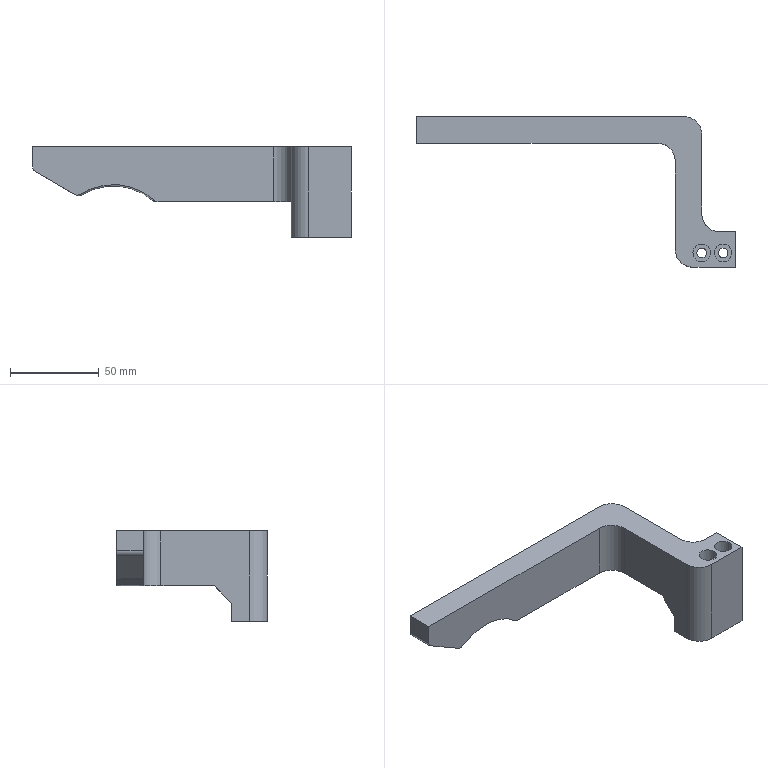Part | NX | 1 solid | 31 faces | box 180 x 85 x 51 mm | volume 114563 mm3 | plane 18 | cylinder 10 | spline 2 | cone 1 | commonest cylinder face diameters 20 x4 5.5 x2 10 x2 6 x1 12.2 x1
STEP:
#1=CARTESIAN_POINT('',(-63.096,27.5,-26.764));
#2=VERTEX_POINT('',#1);
#3=CARTESIAN_POINT('',(-21.145,27.5,-30.228));
#4=VERTEX_POINT('',#3);
#5=CARTESIAN_POINT('',(-44.4,27.5,-56.099));
#6=DIRECTION('',(0.,-1.,0.));
#7=DIRECTION('',(1.,0.,0.));
#8=AXIS2_PLACEMENT_3D('',#5,#6,#7);
#9=CIRCLE('',#8,34.786);
#10=EDGE_CURVE('',#2,#4,#9,.F.);
#11=ORIENTED_EDGE('',*,*,#10,.T.);
#12=CARTESIAN_POINT('',(-19.13,27.5,-31.));
#13=VERTEX_POINT('',#12);
#14=CARTESIAN_POINT('',(-21.145,27.5,-30.228));
#15=CARTESIAN_POINT('',(-20.592,27.5,-30.725));
#16=CARTESIAN_POINT('',(-19.874,27.5,-31.));
#17=CARTESIAN_POINT('',(-19.13,27.5,-31.));
#18=B_SPLINE_CURVE_WITH_KNOTS('',3,(#14,#15,#16,#17),.UNSPECIFIED.,.F.,.F.,(4,4),(0.,0.002195),.UNSPECIFIED.);
#19=EDGE_CURVE('',#4,#13,#18,.T.);
#20=ORIENTED_EDGE('',*,*,#19,.T.);
#21=CARTESIAN_POINT('',(46.,27.5,-31.));
#22=VERTEX_POINT('',#21);
#23=CARTESIAN_POINT('',(-90.,27.5,-31.));
#24=DIRECTION('',(1.,0.,0.));
#25=VECTOR('',#24,1000.);
#26=LINE('',#23,#25);
#27=EDGE_CURVE('',#22,#13,#26,.F.);
#28=ORIENTED_EDGE('',*,*,#27,.F.);
#29=CARTESIAN_POINT('',(46.,27.5,0.));
#30=VERTEX_POINT('',#29);
#31=CARTESIAN_POINT('',(46.,27.5,-31.));
#32=DIRECTION('',(0.,0.,1.));
#33=VECTOR('',#32,1000.);
#34=LINE('',#31,#33);
#35=EDGE_CURVE('',#30,#22,#34,.F.);
#36=ORIENTED_EDGE('',*,*,#35,.F.);
#37=CARTESIAN_POINT('',(-90.,27.5,0.));
#38=VERTEX_POINT('',#37);
#39=CARTESIAN_POINT('',(-20.212,27.5,0.));
#40=DIRECTION('',(1.,0.,0.));
#41=VECTOR('',#40,1000.);
#42=LINE('',#39,#41);
#43=EDGE_CURVE('',#30,#38,#42,.F.);
#44=ORIENTED_EDGE('',*,*,#43,.T.);
#45=CARTESIAN_POINT('',(-90.,27.5,-11.367));
#46=VERTEX_POINT('',#45);
#47=CARTESIAN_POINT('',(-90.,27.5,-31.));
#48=DIRECTION('',(0.,0.,1.));
#49=VECTOR('',#48,1000.);
#50=LINE('',#47,#49);
#51=EDGE_CURVE('',#38,#46,#50,.F.);
#52=ORIENTED_EDGE('',*,*,#51,.T.);
#53=CARTESIAN_POINT('',(-88.5,27.5,-13.965));
#54=VERTEX_POINT('',#53);
#55=CARTESIAN_POINT('',(-87.,27.5,-11.367));
#56=DIRECTION('',(0.,-1.,0.));
#57=DIRECTION('',(1.,0.,0.));
#58=AXIS2_PLACEMENT_3D('',#55,#56,#57);
#59=CIRCLE('',#58,3.);
#60=EDGE_CURVE('',#46,#54,#59,.T.);
#61=ORIENTED_EDGE('',*,*,#60,.T.);
#62=CARTESIAN_POINT('',(-66.215,27.5,-26.831));
#63=VERTEX_POINT('',#62);
#64=CARTESIAN_POINT('',(-29.907,27.5,-47.793));
#65=DIRECTION('',(0.866,0.,-0.5));
#66=VECTOR('',#65,1000.);
#67=LINE('',#64,#66);
#68=EDGE_CURVE('',#54,#63,#67,.T.);
#69=ORIENTED_EDGE('',*,*,#68,.T.);
#70=CARTESIAN_POINT('',(-66.215,27.5,-26.831));
#71=CARTESIAN_POINT('',(-65.26,27.5,-27.383));
#72=CARTESIAN_POINT('',(-64.026,27.5,-27.357));
#73=CARTESIAN_POINT('',(-63.096,27.5,-26.764));
#74=B_SPLINE_CURVE_WITH_KNOTS('',3,(#70,#71,#72,#73),.UNSPECIFIED.,.F.,.F.,(4,4),(0.,0.003262),.UNSPECIFIED.);
#75=EDGE_CURVE('',#63,#2,#74,.T.);
#76=ORIENTED_EDGE('',*,*,#75,.T.);
#77=EDGE_LOOP('',(#11,#20,#28,#36,#44,#52,#61,#69,#76));
#78=FACE_BOUND('',#77,.T.);
#79=CARTESIAN_POINT('',(-20.212,27.5,-31.));
#80=DIRECTION('',(0.,-1.,0.));
#81=DIRECTION('',(0.,0.,-1.));
#82=AXIS2_PLACEMENT_3D('',#79,#80,#81);
#83=PLANE('',#82);
#84=ADVANCED_FACE('',(#78),#83,.T.);
#85=CARTESIAN_POINT('',(-20.322,42.5,-31.));
#86=VERTEX_POINT('',#85);
#87=CARTESIAN_POINT('',(61.,42.5,-31.));
#88=VERTEX_POINT('',#87);
#89=CARTESIAN_POINT('',(61.,42.5,-31.));
#90=DIRECTION('',(-1.,0.,0.));
#91=VECTOR('',#90,1000.);
#92=LINE('',#89,#91);
#93=EDGE_CURVE('',#86,#88,#92,.F.);
#94=ORIENTED_EDGE('',*,*,#93,.F.);
#95=CARTESIAN_POINT('',(-22.283,42.5,-30.275));
#96=VERTEX_POINT('',#95);
#97=CARTESIAN_POINT('',(-20.322,42.5,-31.));
#98=CARTESIAN_POINT('',(-21.041,42.5,-31.));
#99=CARTESIAN_POINT('',(-21.737,42.5,-30.743));
#100=CARTESIAN_POINT('',(-22.283,42.5,-30.275));
#101=B_SPLINE_CURVE_WITH_KNOTS('',3,(#97,#98,#99,#100),.UNSPECIFIED.,.F.,.F.,(4,4),(0.,0.002124),.UNSPECIFIED.);
#102=EDGE_CURVE('',#86,#96,#101,.T.);
#103=ORIENTED_EDGE('',*,*,#102,.T.);
#104=CARTESIAN_POINT('',(-62.355,42.5,-27.226));
#105=VERTEX_POINT('',#104);
#106=CARTESIAN_POINT('',(-44.4,42.5,-56.099));
#107=DIRECTION('',(0.,1.,0.));
#108=DIRECTION('',(-1.,0.,0.));
#109=AXIS2_PLACEMENT_3D('',#106,#107,#108);
#110=CIRCLE('',#109,34.);
#111=EDGE_CURVE('',#96,#105,#110,.F.);
#112=ORIENTED_EDGE('',*,*,#111,.T.);
#113=CARTESIAN_POINT('',(-65.445,42.5,-27.276));
#114=VERTEX_POINT('',#113);
#115=CARTESIAN_POINT('',(-62.355,42.5,-27.226));
#116=CARTESIAN_POINT('',(-63.282,42.5,-27.803));
#117=CARTESIAN_POINT('',(-64.5,42.5,-27.822));
#118=CARTESIAN_POINT('',(-65.445,42.5,-27.276));
#119=B_SPLINE_CURVE_WITH_KNOTS('',3,(#115,#116,#117,#118),.UNSPECIFIED.,.F.,.F.,(4,4),(0.,0.003229),.UNSPECIFIED.);
#120=EDGE_CURVE('',#105,#114,#119,.T.);
#121=ORIENTED_EDGE('',*,*,#120,.T.);
#122=CARTESIAN_POINT('',(-88.5,42.5,-13.965));
#123=VERTEX_POINT('',#122);
#124=CARTESIAN_POINT('',(-66.211,42.5,-26.834));
#125=DIRECTION('',(-0.866,0.,0.5));
#126=VECTOR('',#125,1000.);
#127=LINE('',#124,#126);
#128=EDGE_CURVE('',#114,#123,#127,.T.);
#129=ORIENTED_EDGE('',*,*,#128,.T.);
#130=CARTESIAN_POINT('',(-90.,42.5,-11.367));
#131=VERTEX_POINT('',#130);
#132=CARTESIAN_POINT('',(-87.,42.5,-11.367));
#133=DIRECTION('',(0.,1.,0.));
#134=DIRECTION('',(1.,0.,0.));
#135=AXIS2_PLACEMENT_3D('',#132,#133,#134);
#136=CIRCLE('',#135,3.);
#137=EDGE_CURVE('',#123,#131,#136,.T.);
#138=ORIENTED_EDGE('',*,*,#137,.T.);
#139=CARTESIAN_POINT('',(-90.,42.5,0.));
#140=VERTEX_POINT('',#139);
#141=CARTESIAN_POINT('',(-90.,42.5,-31.));
#142=DIRECTION('',(0.,0.,1.));
#143=VECTOR('',#142,1000.);
#144=LINE('',#141,#143);
#145=EDGE_CURVE('',#140,#131,#144,.F.);
#146=ORIENTED_EDGE('',*,*,#145,.F.);
#147=CARTESIAN_POINT('',(61.,42.5,0.));
#148=VERTEX_POINT('',#147);
#149=CARTESIAN_POINT('',(-88.5,42.5,0.));
#150=DIRECTION('',(-1.,0.,0.));
#151=VECTOR('',#150,1000.);
#152=LINE('',#149,#151);
#153=EDGE_CURVE('',#140,#148,#152,.F.);
#154=ORIENTED_EDGE('',*,*,#153,.T.);
#155=CARTESIAN_POINT('',(61.,42.5,-31.));
#156=DIRECTION('',(0.,0.,1.));
#157=VECTOR('',#156,1000.);
#158=LINE('',#155,#157);
#159=EDGE_CURVE('',#148,#88,#158,.F.);
#160=ORIENTED_EDGE('',*,*,#159,.T.);
#161=EDGE_LOOP('',(#94,#103,#112,#121,#129,#138,#146,#154,#160));
#162=FACE_BOUND('',#161,.T.);
#163=CARTESIAN_POINT('',(-88.5,42.5,-31.));
#164=DIRECTION('',(0.,1.,0.));
#165=DIRECTION('',(0.,0.,1.));
#166=AXIS2_PLACEMENT_3D('',#163,#164,#165);
#167=PLANE('',#166);
#168=ADVANCED_FACE('',(#162),#167,.T.);
#169=CARTESIAN_POINT('',(71.,32.5,-31.));
#170=VERTEX_POINT('',#169);
#171=CARTESIAN_POINT('',(71.,-12.5,-31.));
#172=VERTEX_POINT('',#171);
#173=CARTESIAN_POINT('',(71.,-12.5,-31.));
#174=DIRECTION('',(0.,1.,0.));
#175=VECTOR('',#174,1000.);
#176=LINE('',#173,#175);
#177=EDGE_CURVE('',#170,#172,#176,.F.);
#178=ORIENTED_EDGE('',*,*,#177,.T.);
#179=CARTESIAN_POINT('',(56.,-12.5,-31.));
#180=VERTEX_POINT('',#179);
#181=CARTESIAN_POINT('',(46.,-12.5,-31.));
#182=DIRECTION('',(-1.,0.,0.));
#183=VECTOR('',#182,1000.);
#184=LINE('',#181,#183);
#185=EDGE_CURVE('',#172,#180,#184,.T.);
#186=ORIENTED_EDGE('',*,*,#185,.T.);
#187=CARTESIAN_POINT('',(56.,17.5,-31.));
#188=VERTEX_POINT('',#187);
#189=CARTESIAN_POINT('',(56.,17.5,-31.));
#190=DIRECTION('',(0.,-1.,0.));
#191=VECTOR('',#190,1000.);
#192=LINE('',#189,#191);
#193=EDGE_CURVE('',#180,#188,#192,.F.);
#194=ORIENTED_EDGE('',*,*,#193,.T.);
#195=CARTESIAN_POINT('',(46.,17.5,-31.));
#196=DIRECTION('',(0.,0.,-1.));
#197=DIRECTION('',(1.,0.,0.));
#198=AXIS2_PLACEMENT_3D('',#195,#196,#197);
#199=CIRCLE('',#198,10.);
#200=EDGE_CURVE('',#188,#22,#199,.F.);
#201=ORIENTED_EDGE('',*,*,#200,.T.);
#202=ORIENTED_EDGE('',*,*,#27,.T.);
#203=CARTESIAN_POINT('',(-19.13,27.5,-31.));
#204=CARTESIAN_POINT('',(-19.522,32.5,-31.));
#205=CARTESIAN_POINT('',(-19.919,37.5,-31.));
#206=CARTESIAN_POINT('',(-20.322,42.5,-31.));
#207=B_SPLINE_CURVE_WITH_KNOTS('',3,(#203,#204,#205,#206),.UNSPECIFIED.,.F.,.F.,(4,4),(0.,0.01505),.UNSPECIFIED.);
#208=EDGE_CURVE('',#13,#86,#207,.T.);
#209=ORIENTED_EDGE('',*,*,#208,.T.);
#210=ORIENTED_EDGE('',*,*,#93,.T.);
#211=CARTESIAN_POINT('',(61.,32.5,-31.));
#212=DIRECTION('',(0.,0.,1.));
#213=DIRECTION('',(1.,0.,0.));
#214=AXIS2_PLACEMENT_3D('',#211,#212,#213);
#215=CIRCLE('',#214,10.);
#216=EDGE_CURVE('',#88,#170,#215,.F.);
#217=ORIENTED_EDGE('',*,*,#216,.T.);
#218=EDGE_LOOP('',(#178,#186,#194,#201,#202,#209,#210,#217));
#219=FACE_BOUND('',#218,.T.);
#220=CARTESIAN_POINT('',(46.,17.5,-31.));
#221=DIRECTION('',(0.,0.,-1.));
#222=DIRECTION('',(1.,0.,0.));
#223=AXIS2_PLACEMENT_3D('',#220,#221,#222);
#224=PLANE('',#223);
#225=ADVANCED_FACE('',(#219),#224,.T.);
#226=CARTESIAN_POINT('',(56.,17.5,0.));
#227=VERTEX_POINT('',#226);
#228=CARTESIAN_POINT('',(46.,17.5,0.));
#229=DIRECTION('',(0.,0.,-1.));
#230=DIRECTION('',(1.,0.,0.));
#231=AXIS2_PLACEMENT_3D('',#228,#229,#230);
#232=CIRCLE('',#231,10.);
#233=EDGE_CURVE('',#227,#30,#232,.F.);
#234=ORIENTED_EDGE('',*,*,#233,.T.);
#235=ORIENTED_EDGE('',*,*,#35,.T.);
#236=ORIENTED_EDGE('',*,*,#200,.F.);
#237=CARTESIAN_POINT('',(56.,17.5,-31.));
#238=DIRECTION('',(0.,0.,1.));
#239=VECTOR('',#238,1000.);
#240=LINE('',#237,#239);
#241=EDGE_CURVE('',#227,#188,#240,.F.);
#242=ORIENTED_EDGE('',*,*,#241,.F.);
#243=EDGE_LOOP('',(#234,#235,#236,#242));
#244=FACE_BOUND('',#243,.T.);
#245=CARTESIAN_POINT('',(46.,17.5,-31.));
#246=DIRECTION('',(0.,0.,1.));
#247=DIRECTION('',(-1.,0.,0.));
#248=AXIS2_PLACEMENT_3D('',#245,#246,#247);
#249=CYLINDRICAL_SURFACE('',#248,10.);
#250=ADVANCED_FACE('',(#244),#249,.F.);
#251=CARTESIAN_POINT('',(56.,-32.5,0.));
#252=VERTEX_POINT('',#251);
#253=CARTESIAN_POINT('',(56.,-12.5,0.));
#254=DIRECTION('',(0.,-1.,0.));
#255=VECTOR('',#254,1000.);
#256=LINE('',#253,#255);
#257=EDGE_CURVE('',#252,#227,#256,.F.);
#258=ORIENTED_EDGE('',*,*,#257,.T.);
#259=ORIENTED_EDGE('',*,*,#241,.T.);
#260=ORIENTED_EDGE('',*,*,#193,.F.);
#261=CARTESIAN_POINT('',(56.,-22.5,-41.));
#262=VERTEX_POINT('',#261);
#263=CARTESIAN_POINT('',(56.,-12.5,-31.));
#264=DIRECTION('',(0.,-0.7071,-0.7071));
#265=VECTOR('',#264,1000.);
#266=LINE('',#263,#265);
#267=EDGE_CURVE('',#180,#262,#266,.T.);
#268=ORIENTED_EDGE('',*,*,#267,.T.);
#269=CARTESIAN_POINT('',(56.,-22.5,-51.));
#270=VERTEX_POINT('',#269);
#271=CARTESIAN_POINT('',(56.,-22.5,-51.));
#272=DIRECTION('',(0.,0.,1.));
#273=VECTOR('',#272,1000.);
#274=LINE('',#271,#273);
#275=EDGE_CURVE('',#270,#262,#274,.T.);
#276=ORIENTED_EDGE('',*,*,#275,.F.);
#277=CARTESIAN_POINT('',(56.,-32.5,-51.));
#278=VERTEX_POINT('',#277);
#279=CARTESIAN_POINT('',(56.,-32.5,-51.));
#280=DIRECTION('',(0.,1.,0.));
#281=VECTOR('',#280,1000.);
#282=LINE('',#279,#281);
#283=EDGE_CURVE('',#278,#270,#282,.T.);
#284=ORIENTED_EDGE('',*,*,#283,.F.);
#285=CARTESIAN_POINT('',(56.,-32.5,-51.));
#286=DIRECTION('',(0.,0.,1.));
#287=VECTOR('',#286,1000.);
#288=LINE('',#285,#287);
#289=EDGE_CURVE('',#278,#252,#288,.T.);
#290=ORIENTED_EDGE('',*,*,#289,.T.);
#291=EDGE_LOOP('',(#258,#259,#260,#268,#276,#284,#290));
#292=FACE_BOUND('',#291,.T.);
#293=CARTESIAN_POINT('',(56.,-12.5,-31.));
#294=DIRECTION('',(-1.,0.,0.));
#295=DIRECTION('',(0.,0.,-1.));
#296=AXIS2_PLACEMENT_3D('',#293,#294,#295);
#297=PLANE('',#296);
#298=ADVANCED_FACE('',(#292),#297,.T.);
#299=CARTESIAN_POINT('',(71.,-12.5,0.));
#300=VERTEX_POINT('',#299);
#301=CARTESIAN_POINT('',(81.,-22.5,0.));
#302=VERTEX_POINT('',#301);
#303=CARTESIAN_POINT('',(81.,-12.5,0.));
#304=DIRECTION('',(0.,0.,-1.));
#305=DIRECTION('',(1.,0.,0.));
#306=AXIS2_PLACEMENT_3D('',#303,#304,#305);
#307=CIRCLE('',#306,10.);
#308=EDGE_CURVE('',#300,#302,#307,.F.);
#309=ORIENTED_EDGE('',*,*,#308,.T.);
#310=CARTESIAN_POINT('',(81.,-22.5,-41.));
#311=VERTEX_POINT('',#310);
#312=CARTESIAN_POINT('',(81.,-22.5,-31.));
#313=DIRECTION('',(0.,0.,1.));
#314=VECTOR('',#313,1000.);
#315=LINE('',#312,#314);
#316=EDGE_CURVE('',#302,#311,#315,.F.);
#317=ORIENTED_EDGE('',*,*,#316,.T.);
#318=CARTESIAN_POINT('',(81.,-12.5,-31.));
#319=DIRECTION('',(0.,-0.7071,0.7071));
#320=DIRECTION('',(0.,0.7071,0.7071));
#321=AXIS2_PLACEMENT_3D('',#318,#319,#320);
#322=ELLIPSE('',#321,14.142,10.);
#323=EDGE_CURVE('',#311,#172,#322,.F.);
#324=ORIENTED_EDGE('',*,*,#323,.T.);
#325=CARTESIAN_POINT('',(71.,-12.5,-31.));
#326=DIRECTION('',(0.,0.,1.));
#327=VECTOR('',#326,1000.);
#328=LINE('',#325,#327);
#329=EDGE_CURVE('',#300,#172,#328,.F.);
#330=ORIENTED_EDGE('',*,*,#329,.F.);
#331=EDGE_LOOP('',(#309,#317,#324,#330));
#332=FACE_BOUND('',#331,.T.);
#333=CARTESIAN_POINT('',(81.,-12.5,-31.));
#334=DIRECTION('',(0.,0.,1.));
#335=DIRECTION('',(-1.,0.,0.));
#336=AXIS2_PLACEMENT_3D('',#333,#334,#335);
#337=CYLINDRICAL_SURFACE('',#336,10.);
#338=ADVANCED_FACE('',(#332),#337,.F.);
#339=CARTESIAN_POINT('',(71.,32.5,0.));
#340=VERTEX_POINT('',#339);
#341=CARTESIAN_POINT('',(71.,-12.5,0.));
#342=DIRECTION('',(0.,1.,0.));
#343=VECTOR('',#342,1000.);
#344=LINE('',#341,#343);
#345=EDGE_CURVE('',#340,#300,#344,.F.);
#346=ORIENTED_EDGE('',*,*,#345,.T.);
#347=ORIENTED_EDGE('',*,*,#329,.T.);
#348=ORIENTED_EDGE('',*,*,#177,.F.);
#349=CARTESIAN_POINT('',(71.,32.5,-31.));
#350=DIRECTION('',(0.,0.,1.));
#351=VECTOR('',#350,1000.);
#352=LINE('',#349,#351);
#353=EDGE_CURVE('',#340,#170,#352,.F.);
#354=ORIENTED_EDGE('',*,*,#353,.F.);
#355=EDGE_LOOP('',(#346,#347,#348,#354));
#356=FACE_BOUND('',#355,.T.);
#357=CARTESIAN_POINT('',(71.,-12.5,-31.));
#358=DIRECTION('',(1.,0.,0.));
#359=DIRECTION('',(0.,0.,1.));
#360=AXIS2_PLACEMENT_3D('',#357,#358,#359);
#361=PLANE('',#360);
#362=ADVANCED_FACE('',(#356),#361,.T.);
#363=CARTESIAN_POINT('',(61.,32.5,0.));
#364=DIRECTION('',(0.,0.,1.));
#365=DIRECTION('',(1.,0.,0.));
#366=AXIS2_PLACEMENT_3D('',#363,#364,#365);
#367=CIRCLE('',#366,10.);
#368=EDGE_CURVE('',#148,#340,#367,.F.);
#369=ORIENTED_EDGE('',*,*,#368,.T.);
#370=ORIENTED_EDGE('',*,*,#353,.T.);
#371=ORIENTED_EDGE('',*,*,#216,.F.);
#372=ORIENTED_EDGE('',*,*,#159,.F.);
#373=EDGE_LOOP('',(#369,#370,#371,#372));
#374=FACE_BOUND('',#373,.T.);
#375=CARTESIAN_POINT('',(61.,32.5,-31.));
#376=DIRECTION('',(0.,0.,1.));
#377=DIRECTION('',(-1.,0.,0.));
#378=AXIS2_PLACEMENT_3D('',#375,#376,#377);
#379=CYLINDRICAL_SURFACE('',#378,10.);
#380=ADVANCED_FACE('',(#374),#379,.T.);
#381=CARTESIAN_POINT('',(-90.,-8.5,-11.367));
#382=DIRECTION('',(0.,1.,0.));
#383=VECTOR('',#382,1000.);
#384=LINE('',#381,#383);
#385=EDGE_CURVE('',#46,#131,#384,.T.);
#386=ORIENTED_EDGE('',*,*,#385,.F.);
#387=ORIENTED_EDGE('',*,*,#51,.F.);
#388=CARTESIAN_POINT('',(-90.,42.5,0.));
#389=DIRECTION('',(0.,-1.,0.));
#390=VECTOR('',#389,1000.);
#391=LINE('',#388,#390);
#392=EDGE_CURVE('',#38,#140,#391,.F.);
#393=ORIENTED_EDGE('',*,*,#392,.T.);
#394=ORIENTED_EDGE('',*,*,#145,.T.);
#395=EDGE_LOOP('',(#386,#387,#393,#394));
#396=FACE_BOUND('',#395,.T.);
#397=CARTESIAN_POINT('',(-90.,42.5,-31.));
#398=DIRECTION('',(-1.,0.,0.));
#399=DIRECTION('',(0.,0.,-1.));
#400=AXIS2_PLACEMENT_3D('',#397,#398,#399);
#401=PLANE('',#400);
#402=ADVANCED_FACE('',(#396),#401,.T.);
#403=CARTESIAN_POINT('',(88.,-34.4,0.));
#404=VERTEX_POINT('',#403);
#405=CARTESIAN_POINT('',(83.,-34.4,0.));
#406=DIRECTION('',(0.,0.,-1.));
#407=DIRECTION('',(1.,0.,0.));
#408=AXIS2_PLACEMENT_3D('',#405,#406,#407);
#409=CIRCLE('',#408,5.);
#410=EDGE_CURVE('',#404,#404,#409,.T.);
#411=ORIENTED_EDGE('',*,*,#410,.T.);
#412=EDGE_LOOP('',(#411));
#413=FACE_BOUND('',#412,.T.);
#414=CARTESIAN_POINT('',(76.,-34.4,0.));
#415=VERTEX_POINT('',#414);
#416=CARTESIAN_POINT('',(71.,-34.4,0.));
#417=DIRECTION('',(0.,0.,-1.));
#418=DIRECTION('',(1.,0.,0.));
#419=AXIS2_PLACEMENT_3D('',#416,#417,#418);
#420=CIRCLE('',#419,5.);
#421=EDGE_CURVE('',#415,#415,#420,.T.);
#422=ORIENTED_EDGE('',*,*,#421,.T.);
#423=EDGE_LOOP('',(#422));
#424=FACE_BOUND('',#423,.T.);
#425=ORIENTED_EDGE('',*,*,#392,.F.);
#426=ORIENTED_EDGE('',*,*,#43,.F.);
#427=ORIENTED_EDGE('',*,*,#233,.F.);
#428=ORIENTED_EDGE('',*,*,#257,.F.);
#429=CARTESIAN_POINT('',(66.,-42.5,0.));
#430=VERTEX_POINT('',#429);
#431=CARTESIAN_POINT('',(66.,-32.5,0.));
#432=DIRECTION('',(0.,0.,-1.));
#433=DIRECTION('',(1.,0.,0.));
#434=AXIS2_PLACEMENT_3D('',#431,#432,#433);
#435=CIRCLE('',#434,10.);
#436=EDGE_CURVE('',#430,#252,#435,.T.);
#437=ORIENTED_EDGE('',*,*,#436,.F.);
#438=CARTESIAN_POINT('',(90.,-42.5,0.));
#439=VERTEX_POINT('',#438);
#440=CARTESIAN_POINT('',(90.,-42.5,0.));
#441=DIRECTION('',(-1.,0.,0.));
#442=VECTOR('',#441,1000.);
#443=LINE('',#440,#442);
#444=EDGE_CURVE('',#439,#430,#443,.T.);
#445=ORIENTED_EDGE('',*,*,#444,.F.);
#446=CARTESIAN_POINT('',(90.,-22.5,0.));
#447=VERTEX_POINT('',#446);
#448=CARTESIAN_POINT('',(90.,-40.5,0.));
#449=DIRECTION('',(0.,-1.,0.));
#450=VECTOR('',#449,1000.);
#451=LINE('',#448,#450);
#452=EDGE_CURVE('',#447,#439,#451,.T.);
#453=ORIENTED_EDGE('',*,*,#452,.F.);
#454=CARTESIAN_POINT('',(56.,-22.5,0.));
#455=DIRECTION('',(1.,0.,0.));
#456=VECTOR('',#455,1000.);
#457=LINE('',#454,#456);
#458=EDGE_CURVE('',#302,#447,#457,.T.);
#459=ORIENTED_EDGE('',*,*,#458,.F.);
#460=ORIENTED_EDGE('',*,*,#308,.F.);
#461=ORIENTED_EDGE('',*,*,#345,.F.);
#462=ORIENTED_EDGE('',*,*,#368,.F.);
#463=ORIENTED_EDGE('',*,*,#153,.F.);
#464=EDGE_LOOP('',(#425,#426,#427,#428,#437,#445,#453,#459,#460,#461,#462,#463));
#465=FACE_BOUND('',#464,.T.);
#466=CARTESIAN_POINT('',(46.,17.5,0.));
#467=DIRECTION('',(0.,0.,-1.));
#468=DIRECTION('',(1.,0.,0.));
#469=AXIS2_PLACEMENT_3D('',#466,#467,#468);
#470=PLANE('',#469);
#471=ADVANCED_FACE('',(#413,#424,#465),#470,.F.);
#472=ORIENTED_EDGE('',*,*,#275,.T.);
#473=CARTESIAN_POINT('',(56.,-22.5,-41.));
#474=DIRECTION('',(1.,0.,0.));
#475=VECTOR('',#474,1000.);
#476=LINE('',#473,#475);
#477=EDGE_CURVE('',#262,#311,#476,.T.);
#478=ORIENTED_EDGE('',*,*,#477,.T.);
#479=ORIENTED_EDGE('',*,*,#316,.F.);
#480=ORIENTED_EDGE('',*,*,#458,.T.);
#481=CARTESIAN_POINT('',(90.,-22.5,-51.));
#482=VERTEX_POINT('',#481);
#483=CARTESIAN_POINT('',(90.,-22.5,-51.));
#484=DIRECTION('',(0.,0.,1.));
#485=VECTOR('',#484,1000.);
#486=LINE('',#483,#485);
#487=EDGE_CURVE('',#482,#447,#486,.T.);
#488=ORIENTED_EDGE('',*,*,#487,.F.);
#489=CARTESIAN_POINT('',(56.,-22.5,-51.));
#490=DIRECTION('',(1.,0.,0.));
#491=VECTOR('',#490,1000.);
#492=LINE('',#489,#491);
#493=EDGE_CURVE('',#270,#482,#492,.T.);
#494=ORIENTED_EDGE('',*,*,#493,.F.);
#495=EDGE_LOOP('',(#472,#478,#479,#480,#488,#494));
#496=FACE_BOUND('',#495,.T.);
#497=CARTESIAN_POINT('',(56.,-22.5,-51.));
#498=DIRECTION('',(0.,-1.,0.));
#499=DIRECTION('',(0.,0.,-1.));
#500=AXIS2_PLACEMENT_3D('',#497,#498,#499);
#501=PLANE('',#500);
#502=ADVANCED_FACE('',(#496),#501,.F.);
#503=CARTESIAN_POINT('',(71.,-31.65,-25.8));
#504=VERTEX_POINT('',#503);
#505=CARTESIAN_POINT('',(71.,-34.4,-25.8));
#506=DIRECTION('',(0.,0.,-1.));
#507=DIRECTION('',(0.,1.,0.));
#508=AXIS2_PLACEMENT_3D('',#505,#506,#507);
#509=CIRCLE('',#508,2.75);
#510=EDGE_CURVE('',#504,#504,#509,.T.);
#511=ORIENTED_EDGE('',*,*,#510,.F.);
#512=EDGE_LOOP('',(#511));
#513=FACE_BOUND('',#512,.T.);
#514=CARTESIAN_POINT('',(73.75,-34.4,-35.8));
#515=VERTEX_POINT('',#514);
#516=CARTESIAN_POINT('',(71.,-34.4,-35.8));
#517=DIRECTION('',(0.,0.,-1.));
#518=DIRECTION('',(1.,0.,0.));
#519=AXIS2_PLACEMENT_3D('',#516,#517,#518);
#520=CIRCLE('',#519,2.75);
#521=EDGE_CURVE('',#515,#515,#520,.T.);
#522=ORIENTED_EDGE('',*,*,#521,.T.);
#523=EDGE_LOOP('',(#522));
#524=FACE_BOUND('',#523,.T.);
#525=CARTESIAN_POINT('',(71.,-34.4,-51.));
#526=DIRECTION('',(0.,0.,1.));
#527=DIRECTION('',(-1.,0.,0.));
#528=AXIS2_PLACEMENT_3D('',#525,#526,#527);
#529=CYLINDRICAL_SURFACE('',#528,2.75);
#530=ADVANCED_FACE('',(#513,#524),#529,.F.);
#531=CARTESIAN_POINT('',(83.,-31.65,-25.8));
#532=VERTEX_POINT('',#531);
#533=CARTESIAN_POINT('',(83.,-34.4,-25.8));
#534=DIRECTION('',(0.,0.,-1.));
#535=DIRECTION('',(0.,1.,0.));
#536=AXIS2_PLACEMENT_3D('',#533,#534,#535);
#537=CIRCLE('',#536,2.75);
#538=EDGE_CURVE('',#532,#532,#537,.T.);
#539=ORIENTED_EDGE('',*,*,#538,.F.);
#540=EDGE_LOOP('',(#539));
#541=FACE_BOUND('',#540,.T.);
#542=CARTESIAN_POINT('',(85.75,-34.4,-35.8));
#543=VERTEX_POINT('',#542);
#544=CARTESIAN_POINT('',(83.,-34.4,-35.8));
#545=DIRECTION('',(0.,0.,-1.));
#546=DIRECTION('',(1.,0.,0.));
#547=AXIS2_PLACEMENT_3D('',#544,#545,#546);
#548=CIRCLE('',#547,2.75);
#549=EDGE_CURVE('',#543,#543,#548,.T.);
#550=ORIENTED_EDGE('',*,*,#549,.T.);
#551=EDGE_LOOP('',(#550));
#552=FACE_BOUND('',#551,.T.);
#553=CARTESIAN_POINT('',(83.,-34.4,-51.));
#554=DIRECTION('',(0.,0.,1.));
#555=DIRECTION('',(-1.,0.,0.));
#556=AXIS2_PLACEMENT_3D('',#553,#554,#555);
#557=CYLINDRICAL_SURFACE('',#556,2.75);
#558=ADVANCED_FACE('',(#541,#552),#557,.F.);
#559=ORIENTED_EDGE('',*,*,#444,.T.);
#560=CARTESIAN_POINT('',(66.,-42.5,-51.));
#561=VERTEX_POINT('',#560);
#562=CARTESIAN_POINT('',(66.,-42.5,-51.));
#563=DIRECTION('',(0.,0.,1.));
#564=VECTOR('',#563,1000.);
#565=LINE('',#562,#564);
#566=EDGE_CURVE('',#561,#430,#565,.T.);
#567=ORIENTED_EDGE('',*,*,#566,.F.);
#568=CARTESIAN_POINT('',(90.,-42.5,-51.));
#569=VERTEX_POINT('',#568);
#570=CARTESIAN_POINT('',(90.,-42.5,-51.));
#571=DIRECTION('',(-1.,0.,0.));
#572=VECTOR('',#571,1000.);
#573=LINE('',#570,#572);
#574=EDGE_CURVE('',#569,#561,#573,.T.);
#575=ORIENTED_EDGE('',*,*,#574,.F.);
#576=CARTESIAN_POINT('',(90.,-42.5,-51.));
#577=DIRECTION('',(0.,0.,1.));
#578=VECTOR('',#577,1000.);
#579=LINE('',#576,#578);
#580=EDGE_CURVE('',#569,#439,#579,.T.);
#581=ORIENTED_EDGE('',*,*,#580,.T.);
#582=EDGE_LOOP('',(#559,#567,#575,#581));
#583=FACE_BOUND('',#582,.T.);
#584=CARTESIAN_POINT('',(90.,-42.5,-51.));
#585=DIRECTION('',(0.,1.,0.));
#586=DIRECTION('',(0.,0.,1.));
#587=AXIS2_PLACEMENT_3D('',#584,#585,#586);
#588=PLANE('',#587);
#589=ADVANCED_FACE('',(#583),#588,.F.);
#590=ORIENTED_EDGE('',*,*,#436,.T.);
#591=ORIENTED_EDGE('',*,*,#289,.F.);
#592=CARTESIAN_POINT('',(66.,-32.5,-51.));
#593=DIRECTION('',(0.,0.,-1.));
#594=DIRECTION('',(1.,0.,0.));
#595=AXIS2_PLACEMENT_3D('',#592,#593,#594);
#596=CIRCLE('',#595,10.);
#597=EDGE_CURVE('',#561,#278,#596,.T.);
#598=ORIENTED_EDGE('',*,*,#597,.F.);
#599=ORIENTED_EDGE('',*,*,#566,.T.);
#600=EDGE_LOOP('',(#590,#591,#598,#599));
#601=FACE_BOUND('',#600,.T.);
#602=CARTESIAN_POINT('',(66.,-32.5,-51.));
#603=DIRECTION('',(0.,0.,1.));
#604=DIRECTION('',(-1.,0.,0.));
#605=AXIS2_PLACEMENT_3D('',#602,#603,#604);
#606=CYLINDRICAL_SURFACE('',#605,10.);
#607=ADVANCED_FACE('',(#601),#606,.T.);
#608=CARTESIAN_POINT('',(90.,-40.5,-51.));
#609=VERTEX_POINT('',#608);
#610=CARTESIAN_POINT('',(90.,-22.5,-51.));
#611=DIRECTION('',(0.,-1.,0.));
#612=VECTOR('',#611,1000.);
#613=LINE('',#610,#612);
#614=EDGE_CURVE('',#609,#569,#613,.T.);
#615=ORIENTED_EDGE('',*,*,#614,.F.);
#616=CARTESIAN_POINT('',(90.,-40.5,-35.8));
#617=VERTEX_POINT('',#616);
#618=CARTESIAN_POINT('',(90.,-40.5,-51.));
#619=DIRECTION('',(0.,0.,1.));
#620=VECTOR('',#619,1000.);
#621=LINE('',#618,#620);
#622=EDGE_CURVE('',#609,#617,#621,.T.);
#623=ORIENTED_EDGE('',*,*,#622,.T.);
#624=CARTESIAN_POINT('',(90.,-28.3,-35.8));
#625=VERTEX_POINT('',#624);
#626=CARTESIAN_POINT('',(90.,-28.3,-35.8));
#627=DIRECTION('',(0.,-1.,0.));
#628=VECTOR('',#627,1000.);
#629=LINE('',#626,#628);
#630=EDGE_CURVE('',#625,#617,#629,.T.);
#631=ORIENTED_EDGE('',*,*,#630,.F.);
#632=CARTESIAN_POINT('',(90.,-28.3,-51.));
#633=VERTEX_POINT('',#632);
#634=CARTESIAN_POINT('',(90.,-28.3,-51.));
#635=DIRECTION('',(0.,0.,1.));
#636=VECTOR('',#635,1000.);
#637=LINE('',#634,#636);
#638=EDGE_CURVE('',#633,#625,#637,.T.);
#639=ORIENTED_EDGE('',*,*,#638,.F.);
#640=CARTESIAN_POINT('',(90.,-22.5,-51.));
#641=DIRECTION('',(0.,-1.,0.));
#642=VECTOR('',#641,1000.);
#643=LINE('',#640,#642);
#644=EDGE_CURVE('',#482,#633,#643,.T.);
#645=ORIENTED_EDGE('',*,*,#644,.F.);
#646=ORIENTED_EDGE('',*,*,#487,.T.);
#647=ORIENTED_EDGE('',*,*,#452,.T.);
#648=ORIENTED_EDGE('',*,*,#580,.F.);
#649=EDGE_LOOP('',(#615,#623,#631,#639,#645,#646,#647,#648));
#650=FACE_BOUND('',#649,.T.);
#651=CARTESIAN_POINT('',(90.,-40.5,-51.));
#652=DIRECTION('',(-1.,0.,0.));
#653=DIRECTION('',(0.,0.,-1.));
#654=AXIS2_PLACEMENT_3D('',#651,#652,#653);
#655=PLANE('',#654);
#656=ADVANCED_FACE('',(#650),#655,.F.);
#657=CARTESIAN_POINT('',(64.,-40.5,-51.));
#658=VERTEX_POINT('',#657);
#659=CARTESIAN_POINT('',(90.,-40.5,-51.));
#660=DIRECTION('',(-1.,0.,0.));
#661=VECTOR('',#660,1000.);
#662=LINE('',#659,#661);
#663=EDGE_CURVE('',#609,#658,#662,.T.);
#664=ORIENTED_EDGE('',*,*,#663,.F.);
#665=ORIENTED_EDGE('',*,*,#614,.T.);
#666=ORIENTED_EDGE('',*,*,#574,.T.);
#667=ORIENTED_EDGE('',*,*,#597,.T.);
#668=ORIENTED_EDGE('',*,*,#283,.T.);
#669=ORIENTED_EDGE('',*,*,#493,.T.);
#670=ORIENTED_EDGE('',*,*,#644,.T.);
#671=CARTESIAN_POINT('',(64.,-28.3,-51.));
#672=VERTEX_POINT('',#671);
#673=CARTESIAN_POINT('',(64.,-28.3,-51.));
#674=DIRECTION('',(1.,0.,0.));
#675=VECTOR('',#674,1000.);
#676=LINE('',#673,#675);
#677=EDGE_CURVE('',#672,#633,#676,.T.);
#678=ORIENTED_EDGE('',*,*,#677,.F.);
#679=CARTESIAN_POINT('',(64.,-34.4,-51.));
#680=DIRECTION('',(0.,0.,-1.));
#681=DIRECTION('',(1.,0.,0.));
#682=AXIS2_PLACEMENT_3D('',#679,#680,#681);
#683=CIRCLE('',#682,6.1);
#684=EDGE_CURVE('',#658,#672,#683,.T.);
#685=ORIENTED_EDGE('',*,*,#684,.F.);
#686=EDGE_LOOP('',(#664,#665,#666,#667,#668,#669,#670,#678,#685));
#687=FACE_BOUND('',#686,.T.);
#688=CARTESIAN_POINT('',(66.,-32.5,-51.));
#689=DIRECTION('',(0.,0.,-1.));
#690=DIRECTION('',(1.,0.,0.));
#691=AXIS2_PLACEMENT_3D('',#688,#689,#690);
#692=PLANE('',#691);
#693=ADVANCED_FACE('',(#687),#692,.T.);
#694=CARTESIAN_POINT('',(64.,-40.5,-35.8));
#695=VERTEX_POINT('',#694);
#696=CARTESIAN_POINT('',(90.,-40.5,-35.8));
#697=DIRECTION('',(-1.,0.,0.));
#698=VECTOR('',#697,1000.);
#699=LINE('',#696,#698);
#700=EDGE_CURVE('',#695,#617,#699,.F.);
#701=ORIENTED_EDGE('',*,*,#700,.T.);
#702=ORIENTED_EDGE('',*,*,#622,.F.);
#703=ORIENTED_EDGE('',*,*,#663,.T.);
#704=CARTESIAN_POINT('',(64.,-40.5,-51.));
#705=DIRECTION('',(0.,0.,1.));
#706=VECTOR('',#705,1000.);
#707=LINE('',#704,#706);
#708=EDGE_CURVE('',#695,#658,#707,.F.);
#709=ORIENTED_EDGE('',*,*,#708,.F.);
#710=EDGE_LOOP('',(#701,#702,#703,#709));
#711=FACE_BOUND('',#710,.T.);
#712=CARTESIAN_POINT('',(90.,-40.5,-51.));
#713=DIRECTION('',(0.,1.,0.));
#714=DIRECTION('',(1.,0.,0.));
#715=AXIS2_PLACEMENT_3D('',#712,#713,#714);
#716=PLANE('',#715);
#717=ADVANCED_FACE('',(#711),#716,.T.);
#718=CARTESIAN_POINT('',(64.,-28.3,-35.8));
#719=VERTEX_POINT('',#718);
#720=CARTESIAN_POINT('',(64.,-34.4,-35.8));
#721=DIRECTION('',(0.,0.,-1.));
#722=DIRECTION('',(1.,0.,0.));
#723=AXIS2_PLACEMENT_3D('',#720,#721,#722);
#724=CIRCLE('',#723,6.1);
#725=EDGE_CURVE('',#719,#695,#724,.F.);
#726=ORIENTED_EDGE('',*,*,#725,.T.);
#727=ORIENTED_EDGE('',*,*,#708,.T.);
#728=ORIENTED_EDGE('',*,*,#684,.T.);
#729=CARTESIAN_POINT('',(64.,-28.3,-51.));
#730=DIRECTION('',(0.,0.,1.));
#731=VECTOR('',#730,1000.);
#732=LINE('',#729,#731);
#733=EDGE_CURVE('',#719,#672,#732,.F.);
#734=ORIENTED_EDGE('',*,*,#733,.F.);
#735=EDGE_LOOP('',(#726,#727,#728,#734));
#736=FACE_BOUND('',#735,.T.);
#737=CARTESIAN_POINT('',(64.,-34.4,-51.));
#738=DIRECTION('',(0.,0.,1.));
#739=DIRECTION('',(-1.,0.,0.));
#740=AXIS2_PLACEMENT_3D('',#737,#738,#739);
#741=CYLINDRICAL_SURFACE('',#740,6.1);
#742=ADVANCED_FACE('',(#736),#741,.F.);
#743=CARTESIAN_POINT('',(64.,-28.3,-35.8));
#744=DIRECTION('',(1.,0.,0.));
#745=VECTOR('',#744,1000.);
#746=LINE('',#743,#745);
#747=EDGE_CURVE('',#625,#719,#746,.F.);
#748=ORIENTED_EDGE('',*,*,#747,.T.);
#749=ORIENTED_EDGE('',*,*,#733,.T.);
#750=ORIENTED_EDGE('',*,*,#677,.T.);
#751=ORIENTED_EDGE('',*,*,#638,.T.);
#752=EDGE_LOOP('',(#748,#749,#750,#751));
#753=FACE_BOUND('',#752,.T.);
#754=CARTESIAN_POINT('',(64.,-28.3,-51.));
#755=DIRECTION('',(0.,-1.,0.));
#756=DIRECTION('',(-1.,0.,0.));
#757=AXIS2_PLACEMENT_3D('',#754,#755,#756);
#758=PLANE('',#757);
#759=ADVANCED_FACE('',(#753),#758,.T.);
#760=ORIENTED_EDGE('',*,*,#700,.F.);
#761=ORIENTED_EDGE('',*,*,#725,.F.);
#762=ORIENTED_EDGE('',*,*,#747,.F.);
#763=ORIENTED_EDGE('',*,*,#630,.T.);
#764=EDGE_LOOP('',(#760,#761,#762,#763));
#765=FACE_BOUND('',#764,.T.);
#766=ORIENTED_EDGE('',*,*,#521,.F.);
#767=EDGE_LOOP('',(#766));
#768=FACE_BOUND('',#767,.T.);
#769=ORIENTED_EDGE('',*,*,#549,.F.);
#770=EDGE_LOOP('',(#769));
#771=FACE_BOUND('',#770,.T.);
#772=CARTESIAN_POINT('',(64.,-34.4,-35.8));
#773=DIRECTION('',(0.,0.,-1.));
#774=DIRECTION('',(1.,0.,0.));
#775=AXIS2_PLACEMENT_3D('',#772,#773,#774);
#776=PLANE('',#775);
#777=ADVANCED_FACE('',(#765,#768,#771),#776,.T.);
#778=ORIENTED_EDGE('',*,*,#111,.F.);
#779=CARTESIAN_POINT('',(-22.283,42.5,-30.275));
#780=CARTESIAN_POINT('',(-21.899,37.5,-30.259));
#781=CARTESIAN_POINT('',(-21.52,32.5,-30.244));
#782=CARTESIAN_POINT('',(-21.145,27.5,-30.228));
#783=B_SPLINE_CURVE_WITH_KNOTS('',3,(#779,#780,#781,#782),.UNSPECIFIED.,.F.,.F.,(4,4),(0.,0.01504),.UNSPECIFIED.);
#784=EDGE_CURVE('',#96,#4,#783,.T.);
#785=ORIENTED_EDGE('',*,*,#784,.T.);
#786=ORIENTED_EDGE('',*,*,#10,.F.);
#787=CARTESIAN_POINT('',(-63.096,27.5,-26.764));
#788=CARTESIAN_POINT('',(-62.85,32.5,-26.918));
#789=CARTESIAN_POINT('',(-62.603,37.5,-27.072));
#790=CARTESIAN_POINT('',(-62.355,42.5,-27.226));
#791=B_SPLINE_CURVE_WITH_KNOTS('',3,(#787,#788,#789,#790),.UNSPECIFIED.,.F.,.F.,(4,4),(0.,0.01503),.UNSPECIFIED.);
#792=EDGE_CURVE('',#2,#105,#791,.T.);
#793=ORIENTED_EDGE('',*,*,#792,.T.);
#794=EDGE_LOOP('',(#778,#785,#786,#793));
#795=FACE_BOUND('',#794,.T.);
#796=CARTESIAN_POINT('',(-44.4,42.5,-56.099));
#797=DIRECTION('',(0.,-1.,0.));
#798=DIRECTION('',(-1.,0.,0.));
#799=AXIS2_PLACEMENT_3D('',#796,#797,#798);
#800=CONICAL_SURFACE('',#799,34.,0.05236);
#801=ADVANCED_FACE('',(#795),#800,.F.);
#802=ORIENTED_EDGE('',*,*,#128,.F.);
#803=CARTESIAN_POINT('',(-65.445,42.5,-27.276));
#804=CARTESIAN_POINT('',(-65.702,37.5,-27.127));
#805=CARTESIAN_POINT('',(-65.959,32.5,-26.979));
#806=CARTESIAN_POINT('',(-66.215,27.5,-26.831));
#807=B_SPLINE_CURVE_WITH_KNOTS('',3,(#803,#804,#805,#806),.UNSPECIFIED.,.F.,.F.,(4,4),(0.,0.01503),.UNSPECIFIED.);
#808=EDGE_CURVE('',#114,#63,#807,.T.);
#809=ORIENTED_EDGE('',*,*,#808,.T.);
#810=ORIENTED_EDGE('',*,*,#68,.F.);
#811=CARTESIAN_POINT('',(-88.5,-8.5,-13.965));
#812=DIRECTION('',(0.,1.,0.));
#813=VECTOR('',#812,1000.);
#814=LINE('',#811,#813);
#815=EDGE_CURVE('',#123,#54,#814,.F.);
#816=ORIENTED_EDGE('',*,*,#815,.F.);
#817=EDGE_LOOP('',(#802,#809,#810,#816));
#818=FACE_BOUND('',#817,.T.);
#819=CARTESIAN_POINT('',(-66.211,-8.5,-26.834));
#820=DIRECTION('',(-0.5,0.,-0.866));
#821=DIRECTION('',(0.866,0.,-0.5));
#822=AXIS2_PLACEMENT_3D('',#819,#820,#821);
#823=PLANE('',#822);
#824=ADVANCED_FACE('',(#818),#823,.T.);
#825=ORIENTED_EDGE('',*,*,#385,.T.);
#826=ORIENTED_EDGE('',*,*,#137,.F.);
#827=ORIENTED_EDGE('',*,*,#815,.T.);
#828=ORIENTED_EDGE('',*,*,#60,.F.);
#829=EDGE_LOOP('',(#825,#826,#827,#828));
#830=FACE_BOUND('',#829,.T.);
#831=CARTESIAN_POINT('',(-87.,-8.5,-11.367));
#832=DIRECTION('',(0.,1.,0.));
#833=DIRECTION('',(-1.,0.,0.));
#834=AXIS2_PLACEMENT_3D('',#831,#832,#833);
#835=CYLINDRICAL_SURFACE('',#834,3.);
#836=ADVANCED_FACE('',(#830),#835,.T.);
#837=ORIENTED_EDGE('',*,*,#102,.F.);
#838=ORIENTED_EDGE('',*,*,#208,.F.);
#839=ORIENTED_EDGE('',*,*,#19,.F.);
#840=ORIENTED_EDGE('',*,*,#784,.F.);
#841=EDGE_LOOP('',(#837,#838,#839,#840));
#842=FACE_BOUND('',#841,.T.);
#843=CARTESIAN_POINT('',(-20.342,42.748,-31.));
#844=CARTESIAN_POINT('',(-21.45,42.659,-31.));
#845=CARTESIAN_POINT('',(-22.29,42.591,-30.276));
#846=CARTESIAN_POINT('',(-19.93,37.635,-31.));
#847=CARTESIAN_POINT('',(-21.052,37.538,-31.));
#848=CARTESIAN_POINT('',(-21.898,37.478,-30.259));
#849=CARTESIAN_POINT('',(-19.524,32.522,-31.));
#850=CARTESIAN_POINT('',(-20.66,32.425,-31.));
#851=CARTESIAN_POINT('',(-21.51,32.365,-30.243));
#852=CARTESIAN_POINT('',(-19.123,27.409,-31.));
#853=CARTESIAN_POINT('',(-20.273,27.319,-31.));
#854=CARTESIAN_POINT('',(-21.127,27.252,-30.227));
#855=(BOUNDED_SURFACE()B_SPLINE_SURFACE(3,2,((#843,#844,#845),(#846,#847,#848),(#849,#850,#851),(#852,#853,#854)),.UNSPECIFIED.,.F.,.F.,.F.)B_SPLINE_SURFACE_WITH_KNOTS((4,4),(3,3),(0.06339,0.07877),(0.,1.),.PIECEWISE_BEZIER_KNOTS.)GEOMETRIC_REPRESENTATION_ITEM()RATIONAL_B_SPLINE_SURFACE(((1.,0.9377,1.),(1.,0.9362,1.),(1.,0.9348,1.),(1.,0.9334,1.)))REPRESENTATION_ITEM('')SURFACE());
#856=ADVANCED_FACE('',(#842),#855,.T.);
#857=ORIENTED_EDGE('',*,*,#120,.F.);
#858=ORIENTED_EDGE('',*,*,#792,.F.);
#859=ORIENTED_EDGE('',*,*,#75,.F.);
#860=ORIENTED_EDGE('',*,*,#808,.F.);
#861=EDGE_LOOP('',(#857,#858,#859,#860));
#862=FACE_BOUND('',#861,.T.);
#863=CARTESIAN_POINT('',(-62.35,42.591,-27.229));
#864=CARTESIAN_POINT('',(-63.877,42.641,-28.181));
#865=CARTESIAN_POINT('',(-65.432,42.748,-27.283));
#866=CARTESIAN_POINT('',(-62.604,37.478,-27.071));
#867=CARTESIAN_POINT('',(-64.133,37.522,-28.033));
#868=CARTESIAN_POINT('',(-65.695,37.635,-27.131));
#869=CARTESIAN_POINT('',(-62.856,32.365,-26.914));
#870=CARTESIAN_POINT('',(-64.389,32.409,-27.886));
#871=CARTESIAN_POINT('',(-65.958,32.522,-26.98));
#872=CARTESIAN_POINT('',(-63.109,27.252,-26.757));
#873=CARTESIAN_POINT('',(-64.644,27.302,-27.738));
#874=CARTESIAN_POINT('',(-66.219,27.409,-26.829));
#875=(BOUNDED_SURFACE()B_SPLINE_SURFACE(3,2,((#863,#864,#865),(#866,#867,#868),(#869,#870,#871),(#872,#873,#874)),.UNSPECIFIED.,.F.,.F.,.F.)B_SPLINE_SURFACE_WITH_KNOTS((4,4),(3,3),(0.06343,0.0788),(0.,1.),.PIECEWISE_BEZIER_KNOTS.)GEOMETRIC_REPRESENTATION_ITEM()RATIONAL_B_SPLINE_SURFACE(((1.,0.8576,1.),(1.,0.8566,1.),(1.,0.8556,1.),(1.,0.8546,1.)))REPRESENTATION_ITEM('')SURFACE());
#876=ADVANCED_FACE('',(#862),#875,.T.);
#877=ORIENTED_EDGE('',*,*,#510,.T.);
#878=EDGE_LOOP('',(#877));
#879=FACE_BOUND('',#878,.T.);
#880=CARTESIAN_POINT('',(76.,-34.4,-25.8));
#881=VERTEX_POINT('',#880);
#882=CARTESIAN_POINT('',(71.,-34.4,-25.8));
#883=DIRECTION('',(0.,0.,1.));
#884=DIRECTION('',(1.,0.,0.));
#885=AXIS2_PLACEMENT_3D('',#882,#883,#884);
#886=CIRCLE('',#885,5.);
#887=EDGE_CURVE('',#881,#881,#886,.F.);
#888=ORIENTED_EDGE('',*,*,#887,.F.);
#889=EDGE_LOOP('',(#888));
#890=FACE_BOUND('',#889,.T.);
#891=CARTESIAN_POINT('',(71.,-34.4,-25.8));
#892=DIRECTION('',(0.,0.,-1.));
#893=DIRECTION('',(0.,1.,0.));
#894=AXIS2_PLACEMENT_3D('',#891,#892,#893);
#895=PLANE('',#894);
#896=ADVANCED_FACE('',(#879,#890),#895,.F.);
#897=ORIENTED_EDGE('',*,*,#887,.T.);
#898=EDGE_LOOP('',(#897));
#899=FACE_BOUND('',#898,.T.);
#900=ORIENTED_EDGE('',*,*,#421,.F.);
#901=EDGE_LOOP('',(#900));
#902=FACE_BOUND('',#901,.T.);
#903=CARTESIAN_POINT('',(71.,-34.4,0.));
#904=DIRECTION('',(0.,0.,-1.));
#905=DIRECTION('',(1.,0.,0.));
#906=AXIS2_PLACEMENT_3D('',#903,#904,#905);
#907=CYLINDRICAL_SURFACE('',#906,5.);
#908=ADVANCED_FACE('',(#899,#902),#907,.F.);
#909=ORIENTED_EDGE('',*,*,#538,.T.);
#910=EDGE_LOOP('',(#909));
#911=FACE_BOUND('',#910,.T.);
#912=CARTESIAN_POINT('',(88.,-34.4,-25.8));
#913=VERTEX_POINT('',#912);
#914=CARTESIAN_POINT('',(83.,-34.4,-25.8));
#915=DIRECTION('',(0.,0.,1.));
#916=DIRECTION('',(1.,0.,0.));
#917=AXIS2_PLACEMENT_3D('',#914,#915,#916);
#918=CIRCLE('',#917,5.);
#919=EDGE_CURVE('',#913,#913,#918,.F.);
#920=ORIENTED_EDGE('',*,*,#919,.F.);
#921=EDGE_LOOP('',(#920));
#922=FACE_BOUND('',#921,.T.);
#923=CARTESIAN_POINT('',(83.,-34.4,-25.8));
#924=DIRECTION('',(0.,0.,-1.));
#925=DIRECTION('',(0.,1.,0.));
#926=AXIS2_PLACEMENT_3D('',#923,#924,#925);
#927=PLANE('',#926);
#928=ADVANCED_FACE('',(#911,#922),#927,.F.);
#929=ORIENTED_EDGE('',*,*,#919,.T.);
#930=EDGE_LOOP('',(#929));
#931=FACE_BOUND('',#930,.T.);
#932=ORIENTED_EDGE('',*,*,#410,.F.);
#933=EDGE_LOOP('',(#932));
#934=FACE_BOUND('',#933,.T.);
#935=CARTESIAN_POINT('',(83.,-34.4,0.));
#936=DIRECTION('',(0.,0.,-1.));
#937=DIRECTION('',(1.,0.,0.));
#938=AXIS2_PLACEMENT_3D('',#935,#936,#937);
#939=CYLINDRICAL_SURFACE('',#938,5.);
#940=ADVANCED_FACE('',(#931,#934),#939,.F.);
#941=ORIENTED_EDGE('',*,*,#323,.F.);
#942=ORIENTED_EDGE('',*,*,#477,.F.);
#943=ORIENTED_EDGE('',*,*,#267,.F.);
#944=ORIENTED_EDGE('',*,*,#185,.F.);
#945=EDGE_LOOP('',(#941,#942,#943,#944));
#946=FACE_BOUND('',#945,.T.);
#947=CARTESIAN_POINT('',(46.,-12.5,-31.));
#948=DIRECTION('',(0.,-0.7071,0.7071));
#949=DIRECTION('',(-1.,0.,0.));
#950=AXIS2_PLACEMENT_3D('',#947,#948,#949);
#951=PLANE('',#950);
#952=ADVANCED_FACE('',(#946),#951,.F.);
#953=CLOSED_SHELL('',(#84,#168,#225,#250,#298,#338,#362,#380,#402,#471,#502,#530,#558,#589,#607,#656,#693,#717,#742,#759,#777,#801,#824,#836,#856,#876,#896,#908,#928,#940,#952));
#954=MANIFOLD_SOLID_BREP('',#953);
#955=(LENGTH_UNIT()NAMED_UNIT(*)SI_UNIT(.MILLI.,.METRE.));
#956=UNCERTAINTY_MEASURE_WITH_UNIT(LENGTH_MEASURE(0.0508),#955,'','');
#957=(NAMED_UNIT(*)PLANE_ANGLE_UNIT()SI_UNIT($,.RADIAN.));
#958=(NAMED_UNIT(*)SI_UNIT($,.STERADIAN.)SOLID_ANGLE_UNIT());
#959=(GEOMETRIC_REPRESENTATION_CONTEXT(3)GLOBAL_UNCERTAINTY_ASSIGNED_CONTEXT((#956))GLOBAL_UNIT_ASSIGNED_CONTEXT((#955,#957,#958))REPRESENTATION_CONTEXT('',''));
#960=ADVANCED_BREP_SHAPE_REPRESENTATION('',(#954),#959);